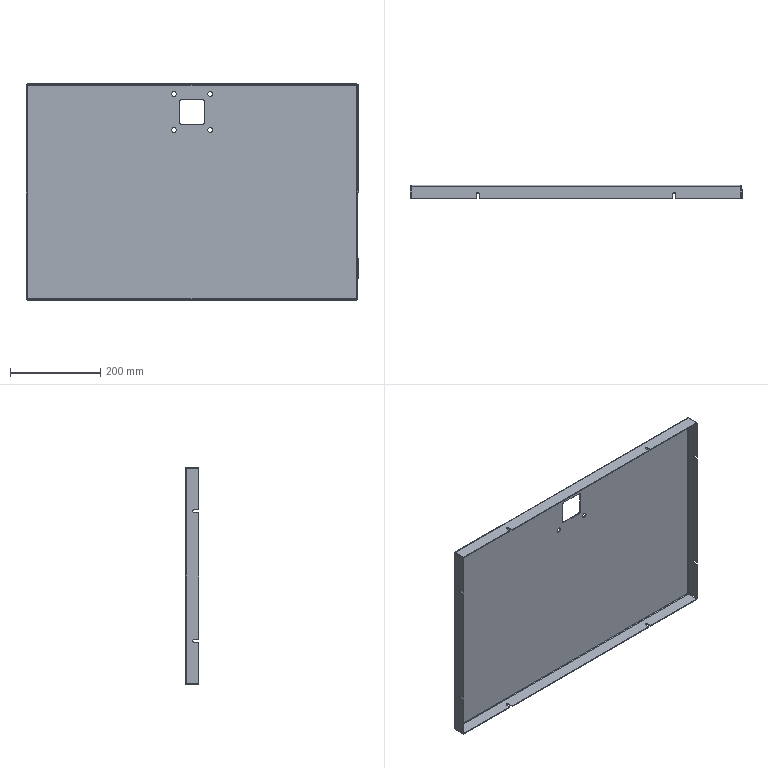Part | STEP file | JBJ-P-1000-18 | 1 solid | 82 faces | box 735 x 30 x 480 mm | volume 827406 mm3 | plane 50 | cylinder 24 | spline 8 | commonest cylinder face diameters 6.5 x8 3 x4 6 x4 7 x4 10.5 x4